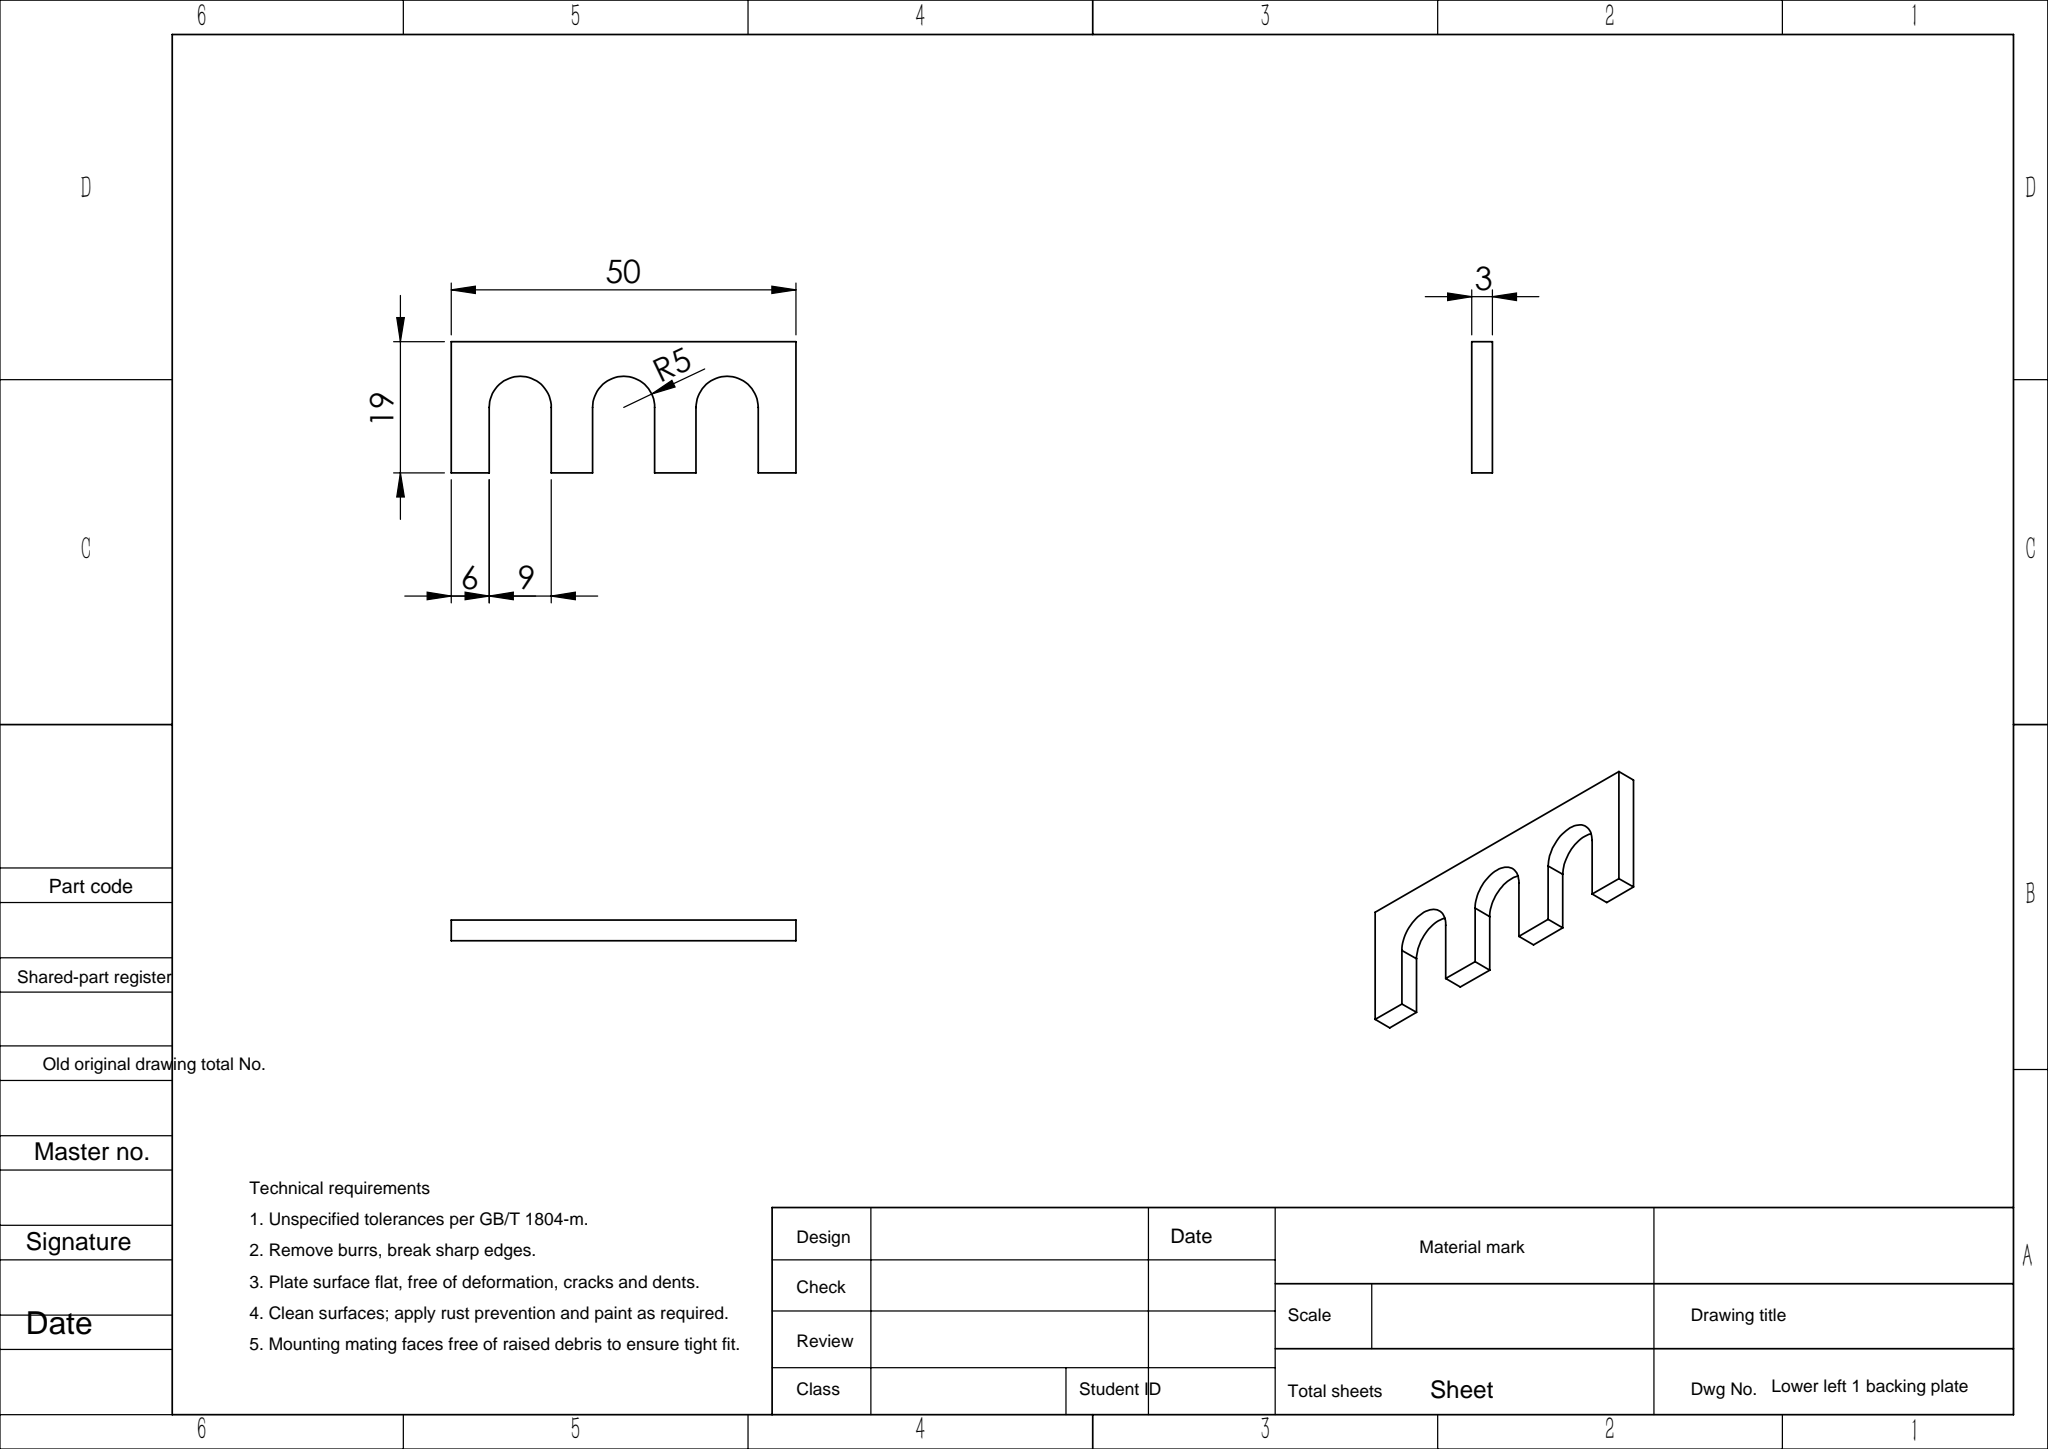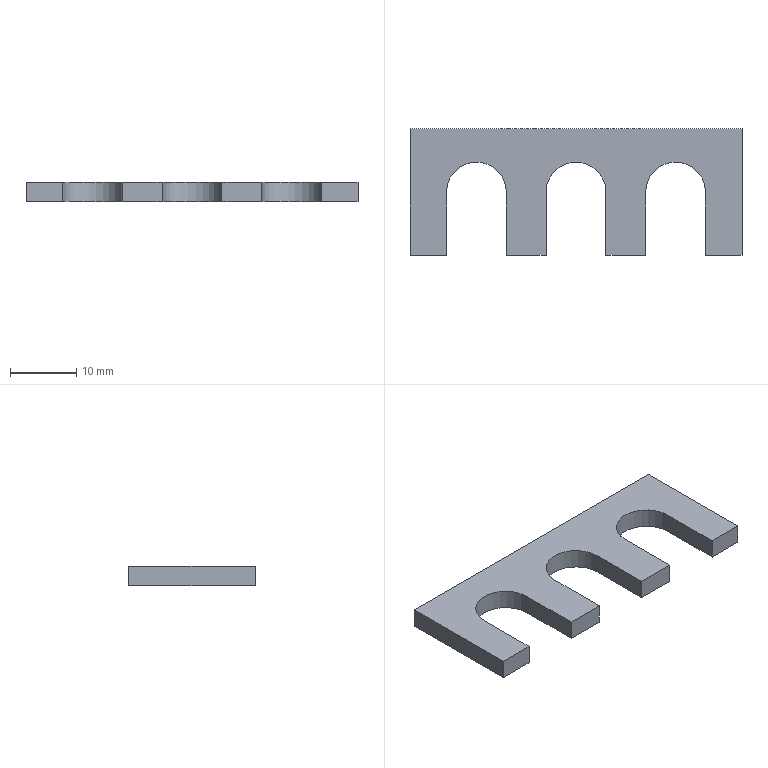Part | SolidWorks | features Extrusion 1 | 1 solid | 18 faces | box 50 x 19 x 3 mm | volume 1794 mm3 | plane 15 | cylinder 3 | commonest cylinder face diameters 9 x3
STEP:
#1=CARTESIAN_POINT('',(0.,19.,0.));
#2=VERTEX_POINT('',#1);
#3=CARTESIAN_POINT('',(0.,0.,0.));
#4=VERTEX_POINT('',#3);
#5=CARTESIAN_POINT('',(0.,0.,0.));
#6=DIRECTION('',(0.,-1.,0.));
#7=VECTOR('',#6,1000.);
#8=LINE('',#5,#7);
#9=EDGE_CURVE('',#2,#4,#8,.T.);
#10=ORIENTED_EDGE('',*,*,#9,.T.);
#11=CARTESIAN_POINT('',(0.,0.,3.));
#12=VERTEX_POINT('',#11);
#13=CARTESIAN_POINT('',(0.,0.,3.));
#14=DIRECTION('',(0.,0.,-1.));
#15=VECTOR('',#14,1000.);
#16=LINE('',#13,#15);
#17=EDGE_CURVE('',#12,#4,#16,.T.);
#18=ORIENTED_EDGE('',*,*,#17,.F.);
#19=CARTESIAN_POINT('',(0.,19.,3.));
#20=VERTEX_POINT('',#19);
#21=CARTESIAN_POINT('',(0.,0.,3.));
#22=DIRECTION('',(0.,-1.,0.));
#23=VECTOR('',#22,1000.);
#24=LINE('',#21,#23);
#25=EDGE_CURVE('',#20,#12,#24,.T.);
#26=ORIENTED_EDGE('',*,*,#25,.F.);
#27=CARTESIAN_POINT('',(0.,19.,3.));
#28=DIRECTION('',(0.,0.,-1.));
#29=VECTOR('',#28,1000.);
#30=LINE('',#27,#29);
#31=EDGE_CURVE('',#20,#2,#30,.T.);
#32=ORIENTED_EDGE('',*,*,#31,.T.);
#33=EDGE_LOOP('',(#10,#18,#26,#32));
#34=FACE_OUTER_BOUND('',#33,.T.);
#35=CARTESIAN_POINT('',(0.,0.,3.));
#36=DIRECTION('',(1.,0.,0.));
#37=DIRECTION('',(0.,0.,-1.));
#38=AXIS2_PLACEMENT_3D('',#35,#36,#37);
#39=PLANE('',#38);
#40=ADVANCED_FACE('',(#34),#39,.F.);
#41=CARTESIAN_POINT('',(5.5,0.,0.));
#42=VERTEX_POINT('',#41);
#43=CARTESIAN_POINT('',(0.,0.,0.));
#44=DIRECTION('',(1.,0.,0.));
#45=VECTOR('',#44,1000.);
#46=LINE('',#43,#45);
#47=EDGE_CURVE('',#4,#42,#46,.T.);
#48=ORIENTED_EDGE('',*,*,#47,.T.);
#49=CARTESIAN_POINT('',(5.5,0.,3.));
#50=VERTEX_POINT('',#49);
#51=CARTESIAN_POINT('',(5.5,0.,3.));
#52=DIRECTION('',(0.,0.,-1.));
#53=VECTOR('',#52,1000.);
#54=LINE('',#51,#53);
#55=EDGE_CURVE('',#50,#42,#54,.T.);
#56=ORIENTED_EDGE('',*,*,#55,.F.);
#57=CARTESIAN_POINT('',(0.,0.,3.));
#58=DIRECTION('',(1.,0.,0.));
#59=VECTOR('',#58,1000.);
#60=LINE('',#57,#59);
#61=EDGE_CURVE('',#12,#50,#60,.T.);
#62=ORIENTED_EDGE('',*,*,#61,.F.);
#63=ORIENTED_EDGE('',*,*,#17,.T.);
#64=EDGE_LOOP('',(#48,#56,#62,#63));
#65=FACE_OUTER_BOUND('',#64,.T.);
#66=CARTESIAN_POINT('',(0.,0.,3.));
#67=DIRECTION('',(0.,1.,0.));
#68=DIRECTION('',(0.,0.,1.));
#69=AXIS2_PLACEMENT_3D('',#66,#67,#68);
#70=PLANE('',#69);
#71=ADVANCED_FACE('',(#65),#70,.F.);
#72=CARTESIAN_POINT('',(5.5,9.5,0.));
#73=VERTEX_POINT('',#72);
#74=CARTESIAN_POINT('',(5.5,9.5,0.));
#75=DIRECTION('',(0.,1.,0.));
#76=VECTOR('',#75,1000.);
#77=LINE('',#74,#76);
#78=EDGE_CURVE('',#42,#73,#77,.T.);
#79=ORIENTED_EDGE('',*,*,#78,.T.);
#80=CARTESIAN_POINT('',(5.5,9.5,3.));
#81=VERTEX_POINT('',#80);
#82=CARTESIAN_POINT('',(5.5,9.5,3.));
#83=DIRECTION('',(0.,0.,-1.));
#84=VECTOR('',#83,1000.);
#85=LINE('',#82,#84);
#86=EDGE_CURVE('',#81,#73,#85,.T.);
#87=ORIENTED_EDGE('',*,*,#86,.F.);
#88=CARTESIAN_POINT('',(5.5,9.5,3.));
#89=DIRECTION('',(0.,1.,0.));
#90=VECTOR('',#89,1000.);
#91=LINE('',#88,#90);
#92=EDGE_CURVE('',#50,#81,#91,.T.);
#93=ORIENTED_EDGE('',*,*,#92,.F.);
#94=ORIENTED_EDGE('',*,*,#55,.T.);
#95=EDGE_LOOP('',(#79,#87,#93,#94));
#96=FACE_OUTER_BOUND('',#95,.T.);
#97=CARTESIAN_POINT('',(5.5,9.5,3.));
#98=DIRECTION('',(-1.,0.,0.));
#99=DIRECTION('',(0.,0.,1.));
#100=AXIS2_PLACEMENT_3D('',#97,#98,#99);
#101=PLANE('',#100);
#102=ADVANCED_FACE('',(#96),#101,.F.);
#103=CARTESIAN_POINT('',(14.5,9.5,0.));
#104=VERTEX_POINT('',#103);
#105=CARTESIAN_POINT('',(10.,9.5,0.));
#106=DIRECTION('',(0.,0.,-1.));
#107=DIRECTION('',(1.,0.,0.));
#108=AXIS2_PLACEMENT_3D('',#105,#106,#107);
#109=CIRCLE('',#108,4.5);
#110=EDGE_CURVE('',#73,#104,#109,.T.);
#111=ORIENTED_EDGE('',*,*,#110,.T.);
#112=CARTESIAN_POINT('',(14.5,9.5,3.));
#113=VERTEX_POINT('',#112);
#114=CARTESIAN_POINT('',(14.5,9.5,3.));
#115=DIRECTION('',(0.,0.,-1.));
#116=VECTOR('',#115,1000.);
#117=LINE('',#114,#116);
#118=EDGE_CURVE('',#113,#104,#117,.T.);
#119=ORIENTED_EDGE('',*,*,#118,.F.);
#120=CARTESIAN_POINT('',(10.,9.5,3.));
#121=DIRECTION('',(0.,0.,-1.));
#122=DIRECTION('',(1.,0.,0.));
#123=AXIS2_PLACEMENT_3D('',#120,#121,#122);
#124=CIRCLE('',#123,4.5);
#125=EDGE_CURVE('',#81,#113,#124,.T.);
#126=ORIENTED_EDGE('',*,*,#125,.F.);
#127=ORIENTED_EDGE('',*,*,#86,.T.);
#128=EDGE_LOOP('',(#111,#119,#126,#127));
#129=FACE_OUTER_BOUND('',#128,.T.);
#130=CARTESIAN_POINT('',(10.,9.5,3.));
#131=DIRECTION('',(0.,0.,-1.));
#132=DIRECTION('',(-1.,0.,0.));
#133=AXIS2_PLACEMENT_3D('',#130,#131,#132);
#134=CYLINDRICAL_SURFACE('',#133,4.5);
#135=ADVANCED_FACE('',(#129),#134,.F.);
#136=CARTESIAN_POINT('',(14.5,0.,0.));
#137=VERTEX_POINT('',#136);
#138=CARTESIAN_POINT('',(14.5,0.,0.));
#139=DIRECTION('',(0.,-1.,0.));
#140=VECTOR('',#139,1000.);
#141=LINE('',#138,#140);
#142=EDGE_CURVE('',#104,#137,#141,.T.);
#143=ORIENTED_EDGE('',*,*,#142,.T.);
#144=CARTESIAN_POINT('',(14.5,0.,3.));
#145=VERTEX_POINT('',#144);
#146=CARTESIAN_POINT('',(14.5,0.,3.));
#147=DIRECTION('',(0.,0.,-1.));
#148=VECTOR('',#147,1000.);
#149=LINE('',#146,#148);
#150=EDGE_CURVE('',#145,#137,#149,.T.);
#151=ORIENTED_EDGE('',*,*,#150,.F.);
#152=CARTESIAN_POINT('',(14.5,0.,3.));
#153=DIRECTION('',(0.,-1.,0.));
#154=VECTOR('',#153,1000.);
#155=LINE('',#152,#154);
#156=EDGE_CURVE('',#113,#145,#155,.T.);
#157=ORIENTED_EDGE('',*,*,#156,.F.);
#158=ORIENTED_EDGE('',*,*,#118,.T.);
#159=EDGE_LOOP('',(#143,#151,#157,#158));
#160=FACE_OUTER_BOUND('',#159,.T.);
#161=CARTESIAN_POINT('',(14.5,0.,3.));
#162=DIRECTION('',(1.,0.,0.));
#163=DIRECTION('',(0.,0.,-1.));
#164=AXIS2_PLACEMENT_3D('',#161,#162,#163);
#165=PLANE('',#164);
#166=ADVANCED_FACE('',(#160),#165,.F.);
#167=CARTESIAN_POINT('',(20.5,0.,0.));
#168=VERTEX_POINT('',#167);
#169=CARTESIAN_POINT('',(14.5,0.,0.));
#170=DIRECTION('',(1.,0.,0.));
#171=VECTOR('',#170,1000.);
#172=LINE('',#169,#171);
#173=EDGE_CURVE('',#137,#168,#172,.T.);
#174=ORIENTED_EDGE('',*,*,#173,.T.);
#175=CARTESIAN_POINT('',(20.5,0.,3.));
#176=VERTEX_POINT('',#175);
#177=CARTESIAN_POINT('',(20.5,0.,3.));
#178=DIRECTION('',(0.,0.,-1.));
#179=VECTOR('',#178,1000.);
#180=LINE('',#177,#179);
#181=EDGE_CURVE('',#176,#168,#180,.T.);
#182=ORIENTED_EDGE('',*,*,#181,.F.);
#183=CARTESIAN_POINT('',(14.5,0.,3.));
#184=DIRECTION('',(1.,0.,0.));
#185=VECTOR('',#184,1000.);
#186=LINE('',#183,#185);
#187=EDGE_CURVE('',#145,#176,#186,.T.);
#188=ORIENTED_EDGE('',*,*,#187,.F.);
#189=ORIENTED_EDGE('',*,*,#150,.T.);
#190=EDGE_LOOP('',(#174,#182,#188,#189));
#191=FACE_OUTER_BOUND('',#190,.T.);
#192=CARTESIAN_POINT('',(14.5,0.,3.));
#193=DIRECTION('',(0.,1.,0.));
#194=DIRECTION('',(0.,0.,1.));
#195=AXIS2_PLACEMENT_3D('',#192,#193,#194);
#196=PLANE('',#195);
#197=ADVANCED_FACE('',(#191),#196,.F.);
#198=CARTESIAN_POINT('',(20.5,9.5,0.));
#199=VERTEX_POINT('',#198);
#200=CARTESIAN_POINT('',(20.5,9.5,0.));
#201=DIRECTION('',(0.,1.,0.));
#202=VECTOR('',#201,1000.);
#203=LINE('',#200,#202);
#204=EDGE_CURVE('',#168,#199,#203,.T.);
#205=ORIENTED_EDGE('',*,*,#204,.T.);
#206=CARTESIAN_POINT('',(20.5,9.5,3.));
#207=VERTEX_POINT('',#206);
#208=CARTESIAN_POINT('',(20.5,9.5,3.));
#209=DIRECTION('',(0.,0.,-1.));
#210=VECTOR('',#209,1000.);
#211=LINE('',#208,#210);
#212=EDGE_CURVE('',#207,#199,#211,.T.);
#213=ORIENTED_EDGE('',*,*,#212,.F.);
#214=CARTESIAN_POINT('',(20.5,9.5,3.));
#215=DIRECTION('',(0.,1.,0.));
#216=VECTOR('',#215,1000.);
#217=LINE('',#214,#216);
#218=EDGE_CURVE('',#176,#207,#217,.T.);
#219=ORIENTED_EDGE('',*,*,#218,.F.);
#220=ORIENTED_EDGE('',*,*,#181,.T.);
#221=EDGE_LOOP('',(#205,#213,#219,#220));
#222=FACE_OUTER_BOUND('',#221,.T.);
#223=CARTESIAN_POINT('',(20.5,9.5,3.));
#224=DIRECTION('',(-1.,0.,0.));
#225=DIRECTION('',(0.,0.,1.));
#226=AXIS2_PLACEMENT_3D('',#223,#224,#225);
#227=PLANE('',#226);
#228=ADVANCED_FACE('',(#222),#227,.F.);
#229=CARTESIAN_POINT('',(29.5,9.5,0.));
#230=VERTEX_POINT('',#229);
#231=CARTESIAN_POINT('',(25.,9.5,0.));
#232=DIRECTION('',(0.,0.,-1.));
#233=DIRECTION('',(1.,0.,0.));
#234=AXIS2_PLACEMENT_3D('',#231,#232,#233);
#235=CIRCLE('',#234,4.5);
#236=EDGE_CURVE('',#199,#230,#235,.T.);
#237=ORIENTED_EDGE('',*,*,#236,.T.);
#238=CARTESIAN_POINT('',(29.5,9.5,3.));
#239=VERTEX_POINT('',#238);
#240=CARTESIAN_POINT('',(29.5,9.5,3.));
#241=DIRECTION('',(0.,0.,-1.));
#242=VECTOR('',#241,1000.);
#243=LINE('',#240,#242);
#244=EDGE_CURVE('',#239,#230,#243,.T.);
#245=ORIENTED_EDGE('',*,*,#244,.F.);
#246=CARTESIAN_POINT('',(25.,9.5,3.));
#247=DIRECTION('',(0.,0.,-1.));
#248=DIRECTION('',(1.,0.,0.));
#249=AXIS2_PLACEMENT_3D('',#246,#247,#248);
#250=CIRCLE('',#249,4.5);
#251=EDGE_CURVE('',#207,#239,#250,.T.);
#252=ORIENTED_EDGE('',*,*,#251,.F.);
#253=ORIENTED_EDGE('',*,*,#212,.T.);
#254=EDGE_LOOP('',(#237,#245,#252,#253));
#255=FACE_OUTER_BOUND('',#254,.T.);
#256=CARTESIAN_POINT('',(25.,9.5,3.));
#257=DIRECTION('',(0.,0.,-1.));
#258=DIRECTION('',(-1.,0.,0.));
#259=AXIS2_PLACEMENT_3D('',#256,#257,#258);
#260=CYLINDRICAL_SURFACE('',#259,4.5);
#261=ADVANCED_FACE('',(#255),#260,.F.);
#262=CARTESIAN_POINT('',(29.5,0.,0.));
#263=VERTEX_POINT('',#262);
#264=CARTESIAN_POINT('',(29.5,9.5,0.));
#265=DIRECTION('',(0.,-1.,0.));
#266=VECTOR('',#265,1000.);
#267=LINE('',#264,#266);
#268=EDGE_CURVE('',#230,#263,#267,.T.);
#269=ORIENTED_EDGE('',*,*,#268,.T.);
#270=CARTESIAN_POINT('',(29.5,0.,3.));
#271=VERTEX_POINT('',#270);
#272=CARTESIAN_POINT('',(29.5,0.,3.));
#273=DIRECTION('',(0.,0.,-1.));
#274=VECTOR('',#273,1000.);
#275=LINE('',#272,#274);
#276=EDGE_CURVE('',#271,#263,#275,.T.);
#277=ORIENTED_EDGE('',*,*,#276,.F.);
#278=CARTESIAN_POINT('',(29.5,9.5,3.));
#279=DIRECTION('',(0.,-1.,0.));
#280=VECTOR('',#279,1000.);
#281=LINE('',#278,#280);
#282=EDGE_CURVE('',#239,#271,#281,.T.);
#283=ORIENTED_EDGE('',*,*,#282,.F.);
#284=ORIENTED_EDGE('',*,*,#244,.T.);
#285=EDGE_LOOP('',(#269,#277,#283,#284));
#286=FACE_OUTER_BOUND('',#285,.T.);
#287=CARTESIAN_POINT('',(29.5,9.5,3.));
#288=DIRECTION('',(1.,0.,0.));
#289=DIRECTION('',(0.,0.,-1.));
#290=AXIS2_PLACEMENT_3D('',#287,#288,#289);
#291=PLANE('',#290);
#292=ADVANCED_FACE('',(#286),#291,.F.);
#293=CARTESIAN_POINT('',(35.5,0.,0.));
#294=VERTEX_POINT('',#293);
#295=CARTESIAN_POINT('',(29.5,0.,0.));
#296=DIRECTION('',(1.,0.,0.));
#297=VECTOR('',#296,1000.);
#298=LINE('',#295,#297);
#299=EDGE_CURVE('',#263,#294,#298,.T.);
#300=ORIENTED_EDGE('',*,*,#299,.T.);
#301=CARTESIAN_POINT('',(35.5,0.,3.));
#302=VERTEX_POINT('',#301);
#303=CARTESIAN_POINT('',(35.5,0.,3.));
#304=DIRECTION('',(0.,0.,-1.));
#305=VECTOR('',#304,1000.);
#306=LINE('',#303,#305);
#307=EDGE_CURVE('',#302,#294,#306,.T.);
#308=ORIENTED_EDGE('',*,*,#307,.F.);
#309=CARTESIAN_POINT('',(29.5,0.,3.));
#310=DIRECTION('',(1.,0.,0.));
#311=VECTOR('',#310,1000.);
#312=LINE('',#309,#311);
#313=EDGE_CURVE('',#271,#302,#312,.T.);
#314=ORIENTED_EDGE('',*,*,#313,.F.);
#315=ORIENTED_EDGE('',*,*,#276,.T.);
#316=EDGE_LOOP('',(#300,#308,#314,#315));
#317=FACE_OUTER_BOUND('',#316,.T.);
#318=CARTESIAN_POINT('',(29.5,0.,3.));
#319=DIRECTION('',(0.,1.,0.));
#320=DIRECTION('',(0.,0.,1.));
#321=AXIS2_PLACEMENT_3D('',#318,#319,#320);
#322=PLANE('',#321);
#323=ADVANCED_FACE('',(#317),#322,.F.);
#324=CARTESIAN_POINT('',(35.5,9.5,0.));
#325=VERTEX_POINT('',#324);
#326=CARTESIAN_POINT('',(35.5,9.5,0.));
#327=DIRECTION('',(0.,1.,0.));
#328=VECTOR('',#327,1000.);
#329=LINE('',#326,#328);
#330=EDGE_CURVE('',#294,#325,#329,.T.);
#331=ORIENTED_EDGE('',*,*,#330,.T.);
#332=CARTESIAN_POINT('',(35.5,9.5,3.));
#333=VERTEX_POINT('',#332);
#334=CARTESIAN_POINT('',(35.5,9.5,3.));
#335=DIRECTION('',(0.,0.,-1.));
#336=VECTOR('',#335,1000.);
#337=LINE('',#334,#336);
#338=EDGE_CURVE('',#333,#325,#337,.T.);
#339=ORIENTED_EDGE('',*,*,#338,.F.);
#340=CARTESIAN_POINT('',(35.5,9.5,3.));
#341=DIRECTION('',(0.,1.,0.));
#342=VECTOR('',#341,1000.);
#343=LINE('',#340,#342);
#344=EDGE_CURVE('',#302,#333,#343,.T.);
#345=ORIENTED_EDGE('',*,*,#344,.F.);
#346=ORIENTED_EDGE('',*,*,#307,.T.);
#347=EDGE_LOOP('',(#331,#339,#345,#346));
#348=FACE_OUTER_BOUND('',#347,.T.);
#349=CARTESIAN_POINT('',(35.5,9.5,3.));
#350=DIRECTION('',(-1.,0.,0.));
#351=DIRECTION('',(0.,0.,1.));
#352=AXIS2_PLACEMENT_3D('',#349,#350,#351);
#353=PLANE('',#352);
#354=ADVANCED_FACE('',(#348),#353,.F.);
#355=CARTESIAN_POINT('',(44.5,9.5,0.));
#356=VERTEX_POINT('',#355);
#357=CARTESIAN_POINT('',(40.,9.5,0.));
#358=DIRECTION('',(0.,0.,-1.));
#359=DIRECTION('',(1.,0.,0.));
#360=AXIS2_PLACEMENT_3D('',#357,#358,#359);
#361=CIRCLE('',#360,4.5);
#362=EDGE_CURVE('',#325,#356,#361,.T.);
#363=ORIENTED_EDGE('',*,*,#362,.T.);
#364=CARTESIAN_POINT('',(44.5,9.5,3.));
#365=VERTEX_POINT('',#364);
#366=CARTESIAN_POINT('',(44.5,9.5,3.));
#367=DIRECTION('',(0.,0.,-1.));
#368=VECTOR('',#367,1000.);
#369=LINE('',#366,#368);
#370=EDGE_CURVE('',#365,#356,#369,.T.);
#371=ORIENTED_EDGE('',*,*,#370,.F.);
#372=CARTESIAN_POINT('',(40.,9.5,3.));
#373=DIRECTION('',(0.,0.,-1.));
#374=DIRECTION('',(1.,0.,0.));
#375=AXIS2_PLACEMENT_3D('',#372,#373,#374);
#376=CIRCLE('',#375,4.5);
#377=EDGE_CURVE('',#333,#365,#376,.T.);
#378=ORIENTED_EDGE('',*,*,#377,.F.);
#379=ORIENTED_EDGE('',*,*,#338,.T.);
#380=EDGE_LOOP('',(#363,#371,#378,#379));
#381=FACE_OUTER_BOUND('',#380,.T.);
#382=CARTESIAN_POINT('',(40.,9.5,3.));
#383=DIRECTION('',(0.,0.,-1.));
#384=DIRECTION('',(-1.,0.,0.));
#385=AXIS2_PLACEMENT_3D('',#382,#383,#384);
#386=CYLINDRICAL_SURFACE('',#385,4.5);
#387=ADVANCED_FACE('',(#381),#386,.F.);
#388=CARTESIAN_POINT('',(44.5,0.,0.));
#389=VERTEX_POINT('',#388);
#390=CARTESIAN_POINT('',(44.5,9.5,0.));
#391=DIRECTION('',(0.,-1.,0.));
#392=VECTOR('',#391,1000.);
#393=LINE('',#390,#392);
#394=EDGE_CURVE('',#356,#389,#393,.T.);
#395=ORIENTED_EDGE('',*,*,#394,.T.);
#396=CARTESIAN_POINT('',(44.5,0.,3.));
#397=VERTEX_POINT('',#396);
#398=CARTESIAN_POINT('',(44.5,0.,3.));
#399=DIRECTION('',(0.,0.,-1.));
#400=VECTOR('',#399,1000.);
#401=LINE('',#398,#400);
#402=EDGE_CURVE('',#397,#389,#401,.T.);
#403=ORIENTED_EDGE('',*,*,#402,.F.);
#404=CARTESIAN_POINT('',(44.5,9.5,3.));
#405=DIRECTION('',(0.,-1.,0.));
#406=VECTOR('',#405,1000.);
#407=LINE('',#404,#406);
#408=EDGE_CURVE('',#365,#397,#407,.T.);
#409=ORIENTED_EDGE('',*,*,#408,.F.);
#410=ORIENTED_EDGE('',*,*,#370,.T.);
#411=EDGE_LOOP('',(#395,#403,#409,#410));
#412=FACE_OUTER_BOUND('',#411,.T.);
#413=CARTESIAN_POINT('',(44.5,9.5,3.));
#414=DIRECTION('',(1.,0.,0.));
#415=DIRECTION('',(0.,0.,-1.));
#416=AXIS2_PLACEMENT_3D('',#413,#414,#415);
#417=PLANE('',#416);
#418=ADVANCED_FACE('',(#412),#417,.F.);
#419=CARTESIAN_POINT('',(50.,0.,0.));
#420=VERTEX_POINT('',#419);
#421=CARTESIAN_POINT('',(44.5,0.,0.));
#422=DIRECTION('',(1.,0.,0.));
#423=VECTOR('',#422,1000.);
#424=LINE('',#421,#423);
#425=EDGE_CURVE('',#389,#420,#424,.T.);
#426=ORIENTED_EDGE('',*,*,#425,.T.);
#427=CARTESIAN_POINT('',(50.,0.,3.));
#428=VERTEX_POINT('',#427);
#429=CARTESIAN_POINT('',(50.,0.,3.));
#430=DIRECTION('',(0.,0.,-1.));
#431=VECTOR('',#430,1000.);
#432=LINE('',#429,#431);
#433=EDGE_CURVE('',#428,#420,#432,.T.);
#434=ORIENTED_EDGE('',*,*,#433,.F.);
#435=CARTESIAN_POINT('',(44.5,0.,3.));
#436=DIRECTION('',(1.,0.,0.));
#437=VECTOR('',#436,1000.);
#438=LINE('',#435,#437);
#439=EDGE_CURVE('',#397,#428,#438,.T.);
#440=ORIENTED_EDGE('',*,*,#439,.F.);
#441=ORIENTED_EDGE('',*,*,#402,.T.);
#442=EDGE_LOOP('',(#426,#434,#440,#441));
#443=FACE_OUTER_BOUND('',#442,.T.);
#444=CARTESIAN_POINT('',(44.5,0.,3.));
#445=DIRECTION('',(0.,1.,0.));
#446=DIRECTION('',(0.,0.,1.));
#447=AXIS2_PLACEMENT_3D('',#444,#445,#446);
#448=PLANE('',#447);
#449=ADVANCED_FACE('',(#443),#448,.F.);
#450=CARTESIAN_POINT('',(50.,19.,0.));
#451=VERTEX_POINT('',#450);
#452=CARTESIAN_POINT('',(50.,0.,0.));
#453=DIRECTION('',(0.,1.,0.));
#454=VECTOR('',#453,1000.);
#455=LINE('',#452,#454);
#456=EDGE_CURVE('',#420,#451,#455,.T.);
#457=ORIENTED_EDGE('',*,*,#456,.T.);
#458=CARTESIAN_POINT('',(50.,19.,3.));
#459=VERTEX_POINT('',#458);
#460=CARTESIAN_POINT('',(50.,19.,3.));
#461=DIRECTION('',(0.,0.,-1.));
#462=VECTOR('',#461,1000.);
#463=LINE('',#460,#462);
#464=EDGE_CURVE('',#459,#451,#463,.T.);
#465=ORIENTED_EDGE('',*,*,#464,.F.);
#466=CARTESIAN_POINT('',(50.,0.,3.));
#467=DIRECTION('',(0.,1.,0.));
#468=VECTOR('',#467,1000.);
#469=LINE('',#466,#468);
#470=EDGE_CURVE('',#428,#459,#469,.T.);
#471=ORIENTED_EDGE('',*,*,#470,.F.);
#472=ORIENTED_EDGE('',*,*,#433,.T.);
#473=EDGE_LOOP('',(#457,#465,#471,#472));
#474=FACE_OUTER_BOUND('',#473,.T.);
#475=CARTESIAN_POINT('',(50.,0.,3.));
#476=DIRECTION('',(-1.,0.,0.));
#477=DIRECTION('',(0.,0.,1.));
#478=AXIS2_PLACEMENT_3D('',#475,#476,#477);
#479=PLANE('',#478);
#480=ADVANCED_FACE('',(#474),#479,.F.);
#481=CARTESIAN_POINT('',(0.,19.,0.));
#482=DIRECTION('',(-1.,0.,0.));
#483=VECTOR('',#482,1000.);
#484=LINE('',#481,#483);
#485=EDGE_CURVE('',#451,#2,#484,.T.);
#486=ORIENTED_EDGE('',*,*,#485,.T.);
#487=ORIENTED_EDGE('',*,*,#31,.F.);
#488=CARTESIAN_POINT('',(0.,19.,3.));
#489=DIRECTION('',(-1.,0.,0.));
#490=VECTOR('',#489,1000.);
#491=LINE('',#488,#490);
#492=EDGE_CURVE('',#459,#20,#491,.T.);
#493=ORIENTED_EDGE('',*,*,#492,.F.);
#494=ORIENTED_EDGE('',*,*,#464,.T.);
#495=EDGE_LOOP('',(#486,#487,#493,#494));
#496=FACE_OUTER_BOUND('',#495,.T.);
#497=CARTESIAN_POINT('',(0.,19.,3.));
#498=DIRECTION('',(0.,-1.,0.));
#499=DIRECTION('',(0.,0.,-1.));
#500=AXIS2_PLACEMENT_3D('',#497,#498,#499);
#501=PLANE('',#500);
#502=ADVANCED_FACE('',(#496),#501,.F.);
#503=ORIENTED_EDGE('',*,*,#25,.T.);
#504=ORIENTED_EDGE('',*,*,#61,.T.);
#505=ORIENTED_EDGE('',*,*,#92,.T.);
#506=ORIENTED_EDGE('',*,*,#125,.T.);
#507=ORIENTED_EDGE('',*,*,#156,.T.);
#508=ORIENTED_EDGE('',*,*,#187,.T.);
#509=ORIENTED_EDGE('',*,*,#218,.T.);
#510=ORIENTED_EDGE('',*,*,#251,.T.);
#511=ORIENTED_EDGE('',*,*,#282,.T.);
#512=ORIENTED_EDGE('',*,*,#313,.T.);
#513=ORIENTED_EDGE('',*,*,#344,.T.);
#514=ORIENTED_EDGE('',*,*,#377,.T.);
#515=ORIENTED_EDGE('',*,*,#408,.T.);
#516=ORIENTED_EDGE('',*,*,#439,.T.);
#517=ORIENTED_EDGE('',*,*,#470,.T.);
#518=ORIENTED_EDGE('',*,*,#492,.T.);
#519=EDGE_LOOP('',(#503,#504,#505,#506,#507,#508,#509,#510,#511,#512,#513,#514,#515,#516,#517,#518));
#520=FACE_OUTER_BOUND('',#519,.T.);
#521=CARTESIAN_POINT('',(40.,9.5,3.));
#522=DIRECTION('',(0.,0.,1.));
#523=DIRECTION('',(1.,0.,0.));
#524=AXIS2_PLACEMENT_3D('',#521,#522,#523);
#525=PLANE('',#524);
#526=ADVANCED_FACE('',(#520),#525,.T.);
#527=ORIENTED_EDGE('',*,*,#9,.F.);
#528=ORIENTED_EDGE('',*,*,#485,.F.);
#529=ORIENTED_EDGE('',*,*,#456,.F.);
#530=ORIENTED_EDGE('',*,*,#425,.F.);
#531=ORIENTED_EDGE('',*,*,#394,.F.);
#532=ORIENTED_EDGE('',*,*,#362,.F.);
#533=ORIENTED_EDGE('',*,*,#330,.F.);
#534=ORIENTED_EDGE('',*,*,#299,.F.);
#535=ORIENTED_EDGE('',*,*,#268,.F.);
#536=ORIENTED_EDGE('',*,*,#236,.F.);
#537=ORIENTED_EDGE('',*,*,#204,.F.);
#538=ORIENTED_EDGE('',*,*,#173,.F.);
#539=ORIENTED_EDGE('',*,*,#142,.F.);
#540=ORIENTED_EDGE('',*,*,#110,.F.);
#541=ORIENTED_EDGE('',*,*,#78,.F.);
#542=ORIENTED_EDGE('',*,*,#47,.F.);
#543=EDGE_LOOP('',(#527,#528,#529,#530,#531,#532,#533,#534,#535,#536,#537,#538,#539,#540,#541,#542));
#544=FACE_OUTER_BOUND('',#543,.T.);
#545=CARTESIAN_POINT('',(40.,9.5,0.));
#546=DIRECTION('',(0.,0.,1.));
#547=DIRECTION('',(1.,0.,0.));
#548=AXIS2_PLACEMENT_3D('',#545,#546,#547);
#549=PLANE('',#548);
#550=ADVANCED_FACE('',(#544),#549,.F.);
#551=CLOSED_SHELL('',(#40,#71,#102,#135,#166,#197,#228,#261,#292,#323,#354,#387,#418,#449,#480,#502,#526,#550));
#552=MANIFOLD_SOLID_BREP('',#551);
#553=CARTESIAN_POINT('',(0.,0.,0.));
#554=DIRECTION('',(0.,0.,1.));
#555=DIRECTION('',(1.,0.,0.));
#556=AXIS2_PLACEMENT_3D('',#553,#554,#555);
#557=(LENGTH_UNIT()NAMED_UNIT(*)SI_UNIT(.MILLI.,.METRE.));
#558=UNCERTAINTY_MEASURE_WITH_UNIT(LENGTH_MEASURE(0.00001),#557,'','');
#559=(NAMED_UNIT(*)PLANE_ANGLE_UNIT()SI_UNIT($,.RADIAN.));
#560=(NAMED_UNIT(*)SI_UNIT($,.STERADIAN.)SOLID_ANGLE_UNIT());
#561=(GEOMETRIC_REPRESENTATION_CONTEXT(3)GLOBAL_UNCERTAINTY_ASSIGNED_CONTEXT((#558))GLOBAL_UNIT_ASSIGNED_CONTEXT((#557,#559,#560))REPRESENTATION_CONTEXT('',''));
#562=ADVANCED_BREP_SHAPE_REPRESENTATION('',(#552,#556),#561);